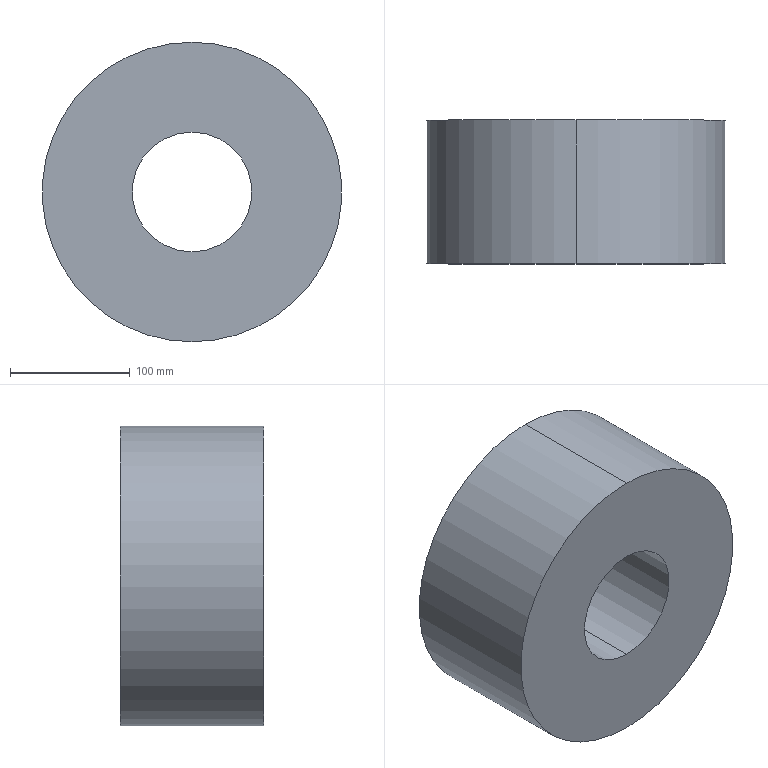Part | SolidWorks | features Extrusion 1 | 1 solid | 6 faces | box 250 x 120 x 250 mm | volume 4948008 mm3 | cylinder 4 | plane 2 | commonest cylinder face diameters 100 x2 250 x2
STEP:
#1=CARTESIAN_POINT('',(0.,60.,-50.));
#2=VERTEX_POINT('',#1);
#3=CARTESIAN_POINT('',(0.,60.,50.));
#4=VERTEX_POINT('',#3);
#5=CARTESIAN_POINT('',(0.,60.,0.));
#6=DIRECTION('',(0.,1.,0.));
#7=DIRECTION('',(0.,0.,1.));
#8=AXIS2_PLACEMENT_3D('',#5,#6,#7);
#9=CIRCLE('',#8,50.);
#10=EDGE_CURVE('',#2,#4,#9,.T.);
#11=ORIENTED_EDGE('',*,*,#10,.T.);
#12=CARTESIAN_POINT('',(0.,-60.,50.));
#13=VERTEX_POINT('',#12);
#14=CARTESIAN_POINT('',(0.,60.,50.));
#15=DIRECTION('',(0.,-1.,0.));
#16=VECTOR('',#15,1000.);
#17=LINE('',#14,#16);
#18=EDGE_CURVE('',#4,#13,#17,.T.);
#19=ORIENTED_EDGE('',*,*,#18,.T.);
#20=CARTESIAN_POINT('',(0.,-60.,-50.));
#21=VERTEX_POINT('',#20);
#22=CARTESIAN_POINT('',(0.,-60.,0.));
#23=DIRECTION('',(0.,1.,0.));
#24=DIRECTION('',(0.,0.,1.));
#25=AXIS2_PLACEMENT_3D('',#22,#23,#24);
#26=CIRCLE('',#25,50.);
#27=EDGE_CURVE('',#21,#13,#26,.T.);
#28=ORIENTED_EDGE('',*,*,#27,.F.);
#29=CARTESIAN_POINT('',(0.,60.,-50.));
#30=DIRECTION('',(0.,-1.,0.));
#31=VECTOR('',#30,1000.);
#32=LINE('',#29,#31);
#33=EDGE_CURVE('',#2,#21,#32,.T.);
#34=ORIENTED_EDGE('',*,*,#33,.F.);
#35=EDGE_LOOP('',(#11,#19,#28,#34));
#36=FACE_OUTER_BOUND('',#35,.T.);
#37=CARTESIAN_POINT('',(0.,60.,0.));
#38=DIRECTION('',(0.,-1.,0.));
#39=DIRECTION('',(0.,0.,-1.));
#40=AXIS2_PLACEMENT_3D('',#37,#38,#39);
#41=CYLINDRICAL_SURFACE('',#40,50.);
#42=ADVANCED_FACE('',(#36),#41,.F.);
#43=CARTESIAN_POINT('',(0.,60.,125.));
#44=VERTEX_POINT('',#43);
#45=CARTESIAN_POINT('',(0.,60.,-125.));
#46=VERTEX_POINT('',#45);
#47=CARTESIAN_POINT('',(0.,60.,0.));
#48=DIRECTION('',(0.,1.,0.));
#49=DIRECTION('',(0.,0.,1.));
#50=AXIS2_PLACEMENT_3D('',#47,#48,#49);
#51=CIRCLE('',#50,125.);
#52=EDGE_CURVE('',#44,#46,#51,.T.);
#53=ORIENTED_EDGE('',*,*,#52,.F.);
#54=CARTESIAN_POINT('',(0.,-60.,125.));
#55=VERTEX_POINT('',#54);
#56=CARTESIAN_POINT('',(0.,60.,125.));
#57=DIRECTION('',(0.,-1.,0.));
#58=VECTOR('',#57,1000.);
#59=LINE('',#56,#58);
#60=EDGE_CURVE('',#44,#55,#59,.T.);
#61=ORIENTED_EDGE('',*,*,#60,.T.);
#62=CARTESIAN_POINT('',(0.,-60.,-125.));
#63=VERTEX_POINT('',#62);
#64=CARTESIAN_POINT('',(0.,-60.,0.));
#65=DIRECTION('',(0.,1.,0.));
#66=DIRECTION('',(0.,0.,1.));
#67=AXIS2_PLACEMENT_3D('',#64,#65,#66);
#68=CIRCLE('',#67,125.);
#69=EDGE_CURVE('',#55,#63,#68,.T.);
#70=ORIENTED_EDGE('',*,*,#69,.T.);
#71=CARTESIAN_POINT('',(0.,60.,-125.));
#72=DIRECTION('',(0.,-1.,0.));
#73=VECTOR('',#72,1000.);
#74=LINE('',#71,#73);
#75=EDGE_CURVE('',#46,#63,#74,.T.);
#76=ORIENTED_EDGE('',*,*,#75,.F.);
#77=EDGE_LOOP('',(#53,#61,#70,#76));
#78=FACE_OUTER_BOUND('',#77,.T.);
#79=CARTESIAN_POINT('',(0.,60.,0.));
#80=DIRECTION('',(0.,-1.,0.));
#81=DIRECTION('',(0.,0.,-1.));
#82=AXIS2_PLACEMENT_3D('',#79,#80,#81);
#83=CYLINDRICAL_SURFACE('',#82,125.);
#84=ADVANCED_FACE('',(#78),#83,.T.);
#85=CARTESIAN_POINT('',(0.,60.,0.));
#86=DIRECTION('',(0.,1.,0.));
#87=DIRECTION('',(0.,0.,1.));
#88=AXIS2_PLACEMENT_3D('',#85,#86,#87);
#89=CIRCLE('',#88,125.);
#90=EDGE_CURVE('',#46,#44,#89,.T.);
#91=ORIENTED_EDGE('',*,*,#90,.T.);
#92=ORIENTED_EDGE('',*,*,#52,.T.);
#93=EDGE_LOOP('',(#91,#92));
#94=FACE_OUTER_BOUND('',#93,.T.);
#95=ORIENTED_EDGE('',*,*,#10,.F.);
#96=CARTESIAN_POINT('',(0.,60.,0.));
#97=DIRECTION('',(0.,1.,0.));
#98=DIRECTION('',(0.,0.,1.));
#99=AXIS2_PLACEMENT_3D('',#96,#97,#98);
#100=CIRCLE('',#99,50.);
#101=EDGE_CURVE('',#4,#2,#100,.T.);
#102=ORIENTED_EDGE('',*,*,#101,.F.);
#103=EDGE_LOOP('',(#95,#102));
#104=FACE_BOUND('',#103,.T.);
#105=CARTESIAN_POINT('',(0.,60.,0.));
#106=DIRECTION('',(0.,1.,0.));
#107=DIRECTION('',(0.,0.,1.));
#108=AXIS2_PLACEMENT_3D('',#105,#106,#107);
#109=PLANE('',#108);
#110=ADVANCED_FACE('',(#94,#104),#109,.T.);
#111=CARTESIAN_POINT('',(0.,-60.,0.));
#112=DIRECTION('',(0.,1.,0.));
#113=DIRECTION('',(0.,0.,1.));
#114=AXIS2_PLACEMENT_3D('',#111,#112,#113);
#115=CIRCLE('',#114,125.);
#116=EDGE_CURVE('',#63,#55,#115,.T.);
#117=ORIENTED_EDGE('',*,*,#116,.F.);
#118=ORIENTED_EDGE('',*,*,#69,.F.);
#119=EDGE_LOOP('',(#117,#118));
#120=FACE_OUTER_BOUND('',#119,.T.);
#121=ORIENTED_EDGE('',*,*,#27,.T.);
#122=CARTESIAN_POINT('',(0.,-60.,0.));
#123=DIRECTION('',(0.,1.,0.));
#124=DIRECTION('',(0.,0.,1.));
#125=AXIS2_PLACEMENT_3D('',#122,#123,#124);
#126=CIRCLE('',#125,50.);
#127=EDGE_CURVE('',#13,#21,#126,.T.);
#128=ORIENTED_EDGE('',*,*,#127,.T.);
#129=EDGE_LOOP('',(#121,#128));
#130=FACE_BOUND('',#129,.T.);
#131=CARTESIAN_POINT('',(0.,-60.,0.));
#132=DIRECTION('',(0.,1.,0.));
#133=DIRECTION('',(0.,0.,1.));
#134=AXIS2_PLACEMENT_3D('',#131,#132,#133);
#135=PLANE('',#134);
#136=ADVANCED_FACE('',(#120,#130),#135,.F.);
#137=ORIENTED_EDGE('',*,*,#60,.F.);
#138=ORIENTED_EDGE('',*,*,#90,.F.);
#139=ORIENTED_EDGE('',*,*,#75,.T.);
#140=ORIENTED_EDGE('',*,*,#116,.T.);
#141=EDGE_LOOP('',(#137,#138,#139,#140));
#142=FACE_OUTER_BOUND('',#141,.T.);
#143=CARTESIAN_POINT('',(0.,60.,0.));
#144=DIRECTION('',(0.,-1.,0.));
#145=DIRECTION('',(0.,0.,-1.));
#146=AXIS2_PLACEMENT_3D('',#143,#144,#145);
#147=CYLINDRICAL_SURFACE('',#146,125.);
#148=ADVANCED_FACE('',(#142),#147,.T.);
#149=ORIENTED_EDGE('',*,*,#18,.F.);
#150=ORIENTED_EDGE('',*,*,#101,.T.);
#151=ORIENTED_EDGE('',*,*,#33,.T.);
#152=ORIENTED_EDGE('',*,*,#127,.F.);
#153=EDGE_LOOP('',(#149,#150,#151,#152));
#154=FACE_OUTER_BOUND('',#153,.T.);
#155=CARTESIAN_POINT('',(0.,60.,0.));
#156=DIRECTION('',(0.,-1.,0.));
#157=DIRECTION('',(0.,0.,-1.));
#158=AXIS2_PLACEMENT_3D('',#155,#156,#157);
#159=CYLINDRICAL_SURFACE('',#158,50.);
#160=ADVANCED_FACE('',(#154),#159,.F.);
#161=CLOSED_SHELL('',(#42,#84,#110,#136,#148,#160));
#162=MANIFOLD_SOLID_BREP('',#161);
#163=CARTESIAN_POINT('',(0.,0.,0.));
#164=DIRECTION('',(0.,0.,1.));
#165=DIRECTION('',(1.,0.,0.));
#166=AXIS2_PLACEMENT_3D('',#163,#164,#165);
#167=(LENGTH_UNIT()NAMED_UNIT(*)SI_UNIT(.MILLI.,.METRE.));
#168=UNCERTAINTY_MEASURE_WITH_UNIT(LENGTH_MEASURE(0.00001),#167,'','');
#169=(NAMED_UNIT(*)PLANE_ANGLE_UNIT()SI_UNIT($,.RADIAN.));
#170=(NAMED_UNIT(*)SI_UNIT($,.STERADIAN.)SOLID_ANGLE_UNIT());
#171=(GEOMETRIC_REPRESENTATION_CONTEXT(3)GLOBAL_UNCERTAINTY_ASSIGNED_CONTEXT((#168))GLOBAL_UNIT_ASSIGNED_CONTEXT((#167,#169,#170))REPRESENTATION_CONTEXT('',''));
#172=ADVANCED_BREP_SHAPE_REPRESENTATION('',(#162,#166),#171);